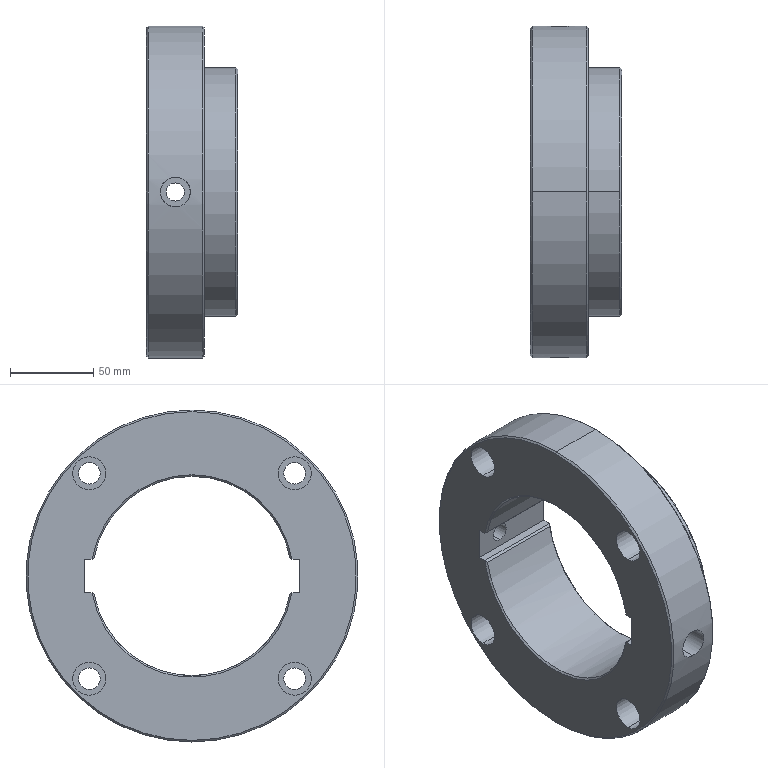Part | SolidWorks | features BaseBody 1 | 1 solid | 62 faces | box 55 x 200 x 200 mm | volume 776397 mm3 | cylinder 31 | plane 19 | cone 12 | commonest cylinder face diameters 13 x8 20 x8 11 x4 18 x4 120 x3 150 x2